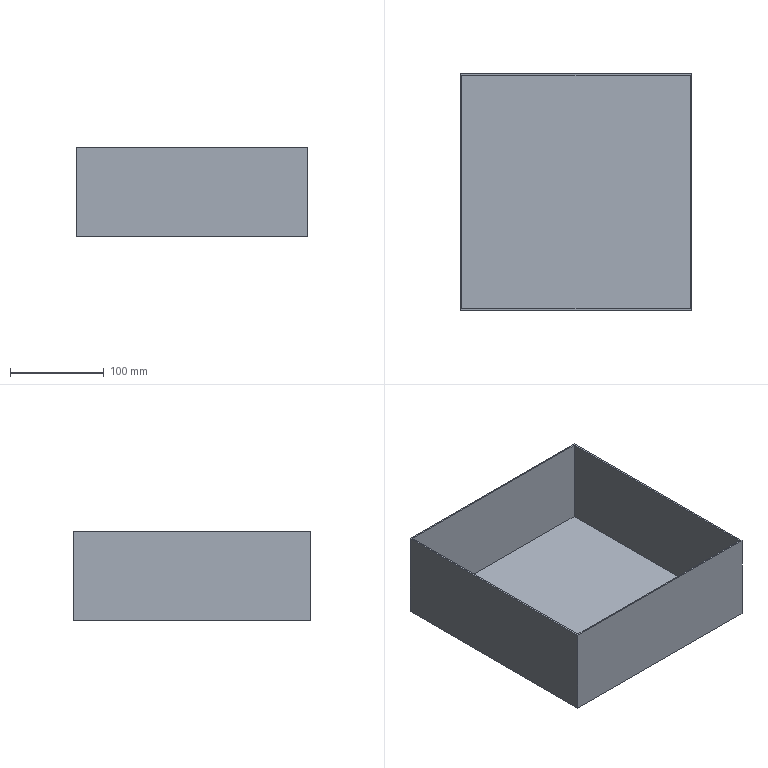Part | STEP file | 012-6-07-012 | 1 solid | 11 faces | box 247 x 253 x 95 mm | volume 309494 mm3 | plane 11
STEP:
#1=CARTESIAN_POINT('',(0.,0.,0.));
#2=DIRECTION('',(0.,0.,1.));
#3=DIRECTION('',(1.,0.,0.));
#4=AXIS2_PLACEMENT_3D('',#1,#2,#3);
#5=CARTESIAN_POINT('',(123.5,-126.5,0.));
#6=VERTEX_POINT('',#5);
#7=CARTESIAN_POINT('',(123.5,126.5,0.));
#8=VERTEX_POINT('',#7);
#9=CARTESIAN_POINT('',(123.5,126.5,0.));
#10=DIRECTION('',(0.,1.,0.));
#11=VECTOR('',#10,1.);
#12=LINE('',#9,#11);
#13=CARTESIAN_POINT('',(123.5,126.5,95.));
#14=DIRECTION('',(-1.,0.,0.));
#15=DIRECTION('',(0.,-1.,0.));
#16=AXIS2_PLACEMENT_3D('',#13,#14,#15);
#17=PLANE('',#16);
#18=CARTESIAN_POINT('',(0.,-95.));
#19=DIRECTION('',(-1.,0.));
#20=VECTOR('',#19,1.);
#21=LINE('',#18,#20);
#22=(GEOMETRIC_REPRESENTATION_CONTEXT(2)PARAMETRIC_REPRESENTATION_CONTEXT()REPRESENTATION_CONTEXT('',''));
#23=DEFINITIONAL_REPRESENTATION('',(#21),#22);
#24=PCURVE('',#17,#23);
#25=CARTESIAN_POINT('',(123.5,-126.5,0.));
#26=DIRECTION('',(0.,0.,1.));
#27=DIRECTION('',(1.,0.,0.));
#28=AXIS2_PLACEMENT_3D('',#25,#26,#27);
#29=PLANE('',#28);
#30=CARTESIAN_POINT('',(0.,253.));
#31=DIRECTION('',(0.,1.));
#32=VECTOR('',#31,1.);
#33=LINE('',#30,#32);
#34=(GEOMETRIC_REPRESENTATION_CONTEXT(2)PARAMETRIC_REPRESENTATION_CONTEXT()REPRESENTATION_CONTEXT('',''));
#35=DEFINITIONAL_REPRESENTATION('',(#33),#34);
#36=PCURVE('',#29,#35);
#37=SURFACE_CURVE('',#12,(#24,#36),.PCURVE_S1.);
#38=EDGE_CURVE('',#6,#8,#37,.T.);
#39=ORIENTED_EDGE('',*,*,#38,.T.);
#40=CARTESIAN_POINT('',(123.5,126.5,95.));
#41=VERTEX_POINT('',#40);
#42=CARTESIAN_POINT('',(123.5,126.5,95.));
#43=DIRECTION('',(0.,0.,-1.));
#44=VECTOR('',#43,1.);
#45=LINE('',#42,#44);
#46=CARTESIAN_POINT('',(0.,0.));
#47=DIRECTION('',(0.,-1.));
#48=VECTOR('',#47,1.);
#49=LINE('',#46,#48);
#50=(GEOMETRIC_REPRESENTATION_CONTEXT(2)PARAMETRIC_REPRESENTATION_CONTEXT()REPRESENTATION_CONTEXT('',''));
#51=DEFINITIONAL_REPRESENTATION('',(#49),#50);
#52=PCURVE('',#17,#51);
#53=CARTESIAN_POINT('',(-123.5,126.5,95.));
#54=DIRECTION('',(0.,-1.,0.));
#55=DIRECTION('',(0.,0.,-1.));
#56=AXIS2_PLACEMENT_3D('',#53,#54,#55);
#57=PLANE('',#56);
#58=CARTESIAN_POINT('',(0.,247.));
#59=DIRECTION('',(1.,0.));
#60=VECTOR('',#59,1.);
#61=LINE('',#58,#60);
#62=(GEOMETRIC_REPRESENTATION_CONTEXT(2)PARAMETRIC_REPRESENTATION_CONTEXT()REPRESENTATION_CONTEXT('',''));
#63=DEFINITIONAL_REPRESENTATION('',(#61),#62);
#64=PCURVE('',#57,#63);
#65=SURFACE_CURVE('',#45,(#52,#64),.PCURVE_S1.);
#66=EDGE_CURVE('',#41,#8,#65,.T.);
#67=ORIENTED_EDGE('',*,*,#66,.F.);
#68=CARTESIAN_POINT('',(123.5,-126.5,95.));
#69=VERTEX_POINT('',#68);
#70=CARTESIAN_POINT('',(123.5,126.5,95.));
#71=DIRECTION('',(0.,1.,0.));
#72=VECTOR('',#71,1.);
#73=LINE('',#70,#72);
#74=CARTESIAN_POINT('',(0.,0.));
#75=DIRECTION('',(-1.,0.));
#76=VECTOR('',#75,1.);
#77=LINE('',#74,#76);
#78=(GEOMETRIC_REPRESENTATION_CONTEXT(2)PARAMETRIC_REPRESENTATION_CONTEXT()REPRESENTATION_CONTEXT('',''));
#79=DEFINITIONAL_REPRESENTATION('',(#77),#78);
#80=PCURVE('',#17,#79);
#81=CARTESIAN_POINT('',(123.5,-126.5,95.));
#82=DIRECTION('',(0.,0.,1.));
#83=DIRECTION('',(1.,0.,0.));
#84=AXIS2_PLACEMENT_3D('',#81,#82,#83);
#85=PLANE('',#84);
#86=CARTESIAN_POINT('',(0.,253.));
#87=DIRECTION('',(0.,1.));
#88=VECTOR('',#87,1.);
#89=LINE('',#86,#88);
#90=(GEOMETRIC_REPRESENTATION_CONTEXT(2)PARAMETRIC_REPRESENTATION_CONTEXT()REPRESENTATION_CONTEXT('',''));
#91=DEFINITIONAL_REPRESENTATION('',(#89),#90);
#92=PCURVE('',#85,#91);
#93=SURFACE_CURVE('',#73,(#80,#92),.PCURVE_S1.);
#94=EDGE_CURVE('',#69,#41,#93,.T.);
#95=ORIENTED_EDGE('',*,*,#94,.F.);
#96=CARTESIAN_POINT('',(123.5,-126.5,95.));
#97=DIRECTION('',(0.,0.,-1.));
#98=VECTOR('',#97,1.);
#99=LINE('',#96,#98);
#100=CARTESIAN_POINT('',(253.,0.));
#101=DIRECTION('',(0.,-1.));
#102=VECTOR('',#101,1.);
#103=LINE('',#100,#102);
#104=(GEOMETRIC_REPRESENTATION_CONTEXT(2)PARAMETRIC_REPRESENTATION_CONTEXT()REPRESENTATION_CONTEXT('',''));
#105=DEFINITIONAL_REPRESENTATION('',(#103),#104);
#106=PCURVE('',#17,#105);
#107=CARTESIAN_POINT('',(-123.5,-126.5,95.));
#108=DIRECTION('',(0.,1.,0.));
#109=DIRECTION('',(0.,0.,1.));
#110=AXIS2_PLACEMENT_3D('',#107,#108,#109);
#111=PLANE('',#110);
#112=CARTESIAN_POINT('',(0.,247.));
#113=DIRECTION('',(-1.,0.));
#114=VECTOR('',#113,1.);
#115=LINE('',#112,#114);
#116=(GEOMETRIC_REPRESENTATION_CONTEXT(2)PARAMETRIC_REPRESENTATION_CONTEXT()REPRESENTATION_CONTEXT('',''));
#117=DEFINITIONAL_REPRESENTATION('',(#115),#116);
#118=PCURVE('',#111,#117);
#119=SURFACE_CURVE('',#99,(#106,#118),.PCURVE_S1.);
#120=EDGE_CURVE('',#69,#6,#119,.T.);
#121=ORIENTED_EDGE('',*,*,#120,.T.);
#122=EDGE_LOOP('',(#39,#67,#95,#121));
#123=FACE_BOUND('',#122,.T.);
#124=ADVANCED_FACE('',(#123),#17,.F.);
#125=CARTESIAN_POINT('',(-123.5,126.5,0.));
#126=VERTEX_POINT('',#125);
#127=CARTESIAN_POINT('',(-123.5,126.5,0.));
#128=DIRECTION('',(-1.,0.,0.));
#129=VECTOR('',#128,1.);
#130=LINE('',#127,#129);
#131=CARTESIAN_POINT('',(95.,0.));
#132=DIRECTION('',(0.,-1.));
#133=VECTOR('',#132,1.);
#134=LINE('',#131,#133);
#135=(GEOMETRIC_REPRESENTATION_CONTEXT(2)PARAMETRIC_REPRESENTATION_CONTEXT()REPRESENTATION_CONTEXT('',''));
#136=DEFINITIONAL_REPRESENTATION('',(#134),#135);
#137=PCURVE('',#57,#136);
#138=CARTESIAN_POINT('',(-247.,253.));
#139=DIRECTION('',(-1.,0.));
#140=VECTOR('',#139,1.);
#141=LINE('',#138,#140);
#142=(GEOMETRIC_REPRESENTATION_CONTEXT(2)PARAMETRIC_REPRESENTATION_CONTEXT()REPRESENTATION_CONTEXT('',''));
#143=DEFINITIONAL_REPRESENTATION('',(#141),#142);
#144=PCURVE('',#29,#143);
#145=SURFACE_CURVE('',#130,(#137,#144),.PCURVE_S1.);
#146=EDGE_CURVE('',#8,#126,#145,.T.);
#147=ORIENTED_EDGE('',*,*,#146,.T.);
#148=CARTESIAN_POINT('',(-123.5,126.5,95.));
#149=VERTEX_POINT('',#148);
#150=CARTESIAN_POINT('',(-123.5,126.5,95.));
#151=DIRECTION('',(0.,0.,-1.));
#152=VECTOR('',#151,1.);
#153=LINE('',#150,#152);
#154=CARTESIAN_POINT('',(0.,0.));
#155=DIRECTION('',(1.,0.));
#156=VECTOR('',#155,1.);
#157=LINE('',#154,#156);
#158=(GEOMETRIC_REPRESENTATION_CONTEXT(2)PARAMETRIC_REPRESENTATION_CONTEXT()REPRESENTATION_CONTEXT('',''));
#159=DEFINITIONAL_REPRESENTATION('',(#157),#158);
#160=PCURVE('',#57,#159);
#161=CARTESIAN_POINT('',(-123.5,126.5,95.));
#162=DIRECTION('',(1.,0.,0.));
#163=DIRECTION('',(0.,1.,0.));
#164=AXIS2_PLACEMENT_3D('',#161,#162,#163);
#165=PLANE('',#164);
#166=CARTESIAN_POINT('',(0.,0.));
#167=DIRECTION('',(0.,-1.));
#168=VECTOR('',#167,1.);
#169=LINE('',#166,#168);
#170=(GEOMETRIC_REPRESENTATION_CONTEXT(2)PARAMETRIC_REPRESENTATION_CONTEXT()REPRESENTATION_CONTEXT('',''));
#171=DEFINITIONAL_REPRESENTATION('',(#169),#170);
#172=PCURVE('',#165,#171);
#173=SURFACE_CURVE('',#153,(#160,#172),.PCURVE_S1.);
#174=EDGE_CURVE('',#149,#126,#173,.T.);
#175=ORIENTED_EDGE('',*,*,#174,.F.);
#176=CARTESIAN_POINT('',(-123.5,126.5,95.));
#177=DIRECTION('',(-1.,0.,0.));
#178=VECTOR('',#177,1.);
#179=LINE('',#176,#178);
#180=CARTESIAN_POINT('',(0.,0.));
#181=DIRECTION('',(0.,-1.));
#182=VECTOR('',#181,1.);
#183=LINE('',#180,#182);
#184=(GEOMETRIC_REPRESENTATION_CONTEXT(2)PARAMETRIC_REPRESENTATION_CONTEXT()REPRESENTATION_CONTEXT('',''));
#185=DEFINITIONAL_REPRESENTATION('',(#183),#184);
#186=PCURVE('',#57,#185);
#187=CARTESIAN_POINT('',(-247.,253.));
#188=DIRECTION('',(-1.,0.));
#189=VECTOR('',#188,1.);
#190=LINE('',#187,#189);
#191=(GEOMETRIC_REPRESENTATION_CONTEXT(2)PARAMETRIC_REPRESENTATION_CONTEXT()REPRESENTATION_CONTEXT('',''));
#192=DEFINITIONAL_REPRESENTATION('',(#190),#191);
#193=PCURVE('',#85,#192);
#194=SURFACE_CURVE('',#179,(#186,#193),.PCURVE_S1.);
#195=EDGE_CURVE('',#41,#149,#194,.T.);
#196=ORIENTED_EDGE('',*,*,#195,.F.);
#197=ORIENTED_EDGE('',*,*,#66,.T.);
#198=EDGE_LOOP('',(#147,#175,#196,#197));
#199=FACE_BOUND('',#198,.T.);
#200=ADVANCED_FACE('',(#199),#57,.F.);
#201=CARTESIAN_POINT('',(-123.5,-126.5,0.));
#202=VERTEX_POINT('',#201);
#203=CARTESIAN_POINT('',(-123.5,126.5,0.));
#204=DIRECTION('',(0.,-1.,0.));
#205=VECTOR('',#204,1.);
#206=LINE('',#203,#205);
#207=CARTESIAN_POINT('',(0.,-95.));
#208=DIRECTION('',(-1.,0.));
#209=VECTOR('',#208,1.);
#210=LINE('',#207,#209);
#211=(GEOMETRIC_REPRESENTATION_CONTEXT(2)PARAMETRIC_REPRESENTATION_CONTEXT()REPRESENTATION_CONTEXT('',''));
#212=DEFINITIONAL_REPRESENTATION('',(#210),#211);
#213=PCURVE('',#165,#212);
#214=CARTESIAN_POINT('',(-247.,253.));
#215=DIRECTION('',(0.,-1.));
#216=VECTOR('',#215,1.);
#217=LINE('',#214,#216);
#218=(GEOMETRIC_REPRESENTATION_CONTEXT(2)PARAMETRIC_REPRESENTATION_CONTEXT()REPRESENTATION_CONTEXT('',''));
#219=DEFINITIONAL_REPRESENTATION('',(#217),#218);
#220=PCURVE('',#29,#219);
#221=SURFACE_CURVE('',#206,(#213,#220),.PCURVE_S1.);
#222=EDGE_CURVE('',#126,#202,#221,.T.);
#223=ORIENTED_EDGE('',*,*,#222,.T.);
#224=CARTESIAN_POINT('',(-123.5,-126.5,95.));
#225=VERTEX_POINT('',#224);
#226=CARTESIAN_POINT('',(-123.5,-126.5,95.));
#227=DIRECTION('',(0.,0.,-1.));
#228=VECTOR('',#227,1.);
#229=LINE('',#226,#228);
#230=CARTESIAN_POINT('',(-253.,0.));
#231=DIRECTION('',(0.,-1.));
#232=VECTOR('',#231,1.);
#233=LINE('',#230,#232);
#234=(GEOMETRIC_REPRESENTATION_CONTEXT(2)PARAMETRIC_REPRESENTATION_CONTEXT()REPRESENTATION_CONTEXT('',''));
#235=DEFINITIONAL_REPRESENTATION('',(#233),#234);
#236=PCURVE('',#165,#235);
#237=CARTESIAN_POINT('',(0.,0.));
#238=DIRECTION('',(-1.,0.));
#239=VECTOR('',#238,1.);
#240=LINE('',#237,#239);
#241=(GEOMETRIC_REPRESENTATION_CONTEXT(2)PARAMETRIC_REPRESENTATION_CONTEXT()REPRESENTATION_CONTEXT('',''));
#242=DEFINITIONAL_REPRESENTATION('',(#240),#241);
#243=PCURVE('',#111,#242);
#244=SURFACE_CURVE('',#229,(#236,#243),.PCURVE_S1.);
#245=EDGE_CURVE('',#225,#202,#244,.T.);
#246=ORIENTED_EDGE('',*,*,#245,.F.);
#247=CARTESIAN_POINT('',(-123.5,126.5,95.));
#248=DIRECTION('',(0.,-1.,0.));
#249=VECTOR('',#248,1.);
#250=LINE('',#247,#249);
#251=CARTESIAN_POINT('',(0.,0.));
#252=DIRECTION('',(-1.,0.));
#253=VECTOR('',#252,1.);
#254=LINE('',#251,#253);
#255=(GEOMETRIC_REPRESENTATION_CONTEXT(2)PARAMETRIC_REPRESENTATION_CONTEXT()REPRESENTATION_CONTEXT('',''));
#256=DEFINITIONAL_REPRESENTATION('',(#254),#255);
#257=PCURVE('',#165,#256);
#258=CARTESIAN_POINT('',(-247.,253.));
#259=DIRECTION('',(0.,-1.));
#260=VECTOR('',#259,1.);
#261=LINE('',#258,#260);
#262=(GEOMETRIC_REPRESENTATION_CONTEXT(2)PARAMETRIC_REPRESENTATION_CONTEXT()REPRESENTATION_CONTEXT('',''));
#263=DEFINITIONAL_REPRESENTATION('',(#261),#262);
#264=PCURVE('',#85,#263);
#265=SURFACE_CURVE('',#250,(#257,#264),.PCURVE_S1.);
#266=EDGE_CURVE('',#149,#225,#265,.T.);
#267=ORIENTED_EDGE('',*,*,#266,.F.);
#268=ORIENTED_EDGE('',*,*,#174,.T.);
#269=EDGE_LOOP('',(#223,#246,#267,#268));
#270=FACE_BOUND('',#269,.T.);
#271=ADVANCED_FACE('',(#270),#165,.F.);
#272=CARTESIAN_POINT('',(-123.5,-126.5,0.));
#273=DIRECTION('',(1.,0.,0.));
#274=VECTOR('',#273,1.);
#275=LINE('',#272,#274);
#276=CARTESIAN_POINT('',(-95.,0.));
#277=DIRECTION('',(0.,1.));
#278=VECTOR('',#277,1.);
#279=LINE('',#276,#278);
#280=(GEOMETRIC_REPRESENTATION_CONTEXT(2)PARAMETRIC_REPRESENTATION_CONTEXT()REPRESENTATION_CONTEXT('',''));
#281=DEFINITIONAL_REPRESENTATION('',(#279),#280);
#282=PCURVE('',#111,#281);
#283=CARTESIAN_POINT('',(-247.,0.));
#284=DIRECTION('',(1.,0.));
#285=VECTOR('',#284,1.);
#286=LINE('',#283,#285);
#287=(GEOMETRIC_REPRESENTATION_CONTEXT(2)PARAMETRIC_REPRESENTATION_CONTEXT()REPRESENTATION_CONTEXT('',''));
#288=DEFINITIONAL_REPRESENTATION('',(#286),#287);
#289=PCURVE('',#29,#288);
#290=SURFACE_CURVE('',#275,(#282,#289),.PCURVE_S1.);
#291=EDGE_CURVE('',#202,#6,#290,.T.);
#292=ORIENTED_EDGE('',*,*,#291,.T.);
#293=ORIENTED_EDGE('',*,*,#120,.F.);
#294=CARTESIAN_POINT('',(-123.5,-126.5,95.));
#295=DIRECTION('',(1.,0.,0.));
#296=VECTOR('',#295,1.);
#297=LINE('',#294,#296);
#298=CARTESIAN_POINT('',(0.,0.));
#299=DIRECTION('',(0.,1.));
#300=VECTOR('',#299,1.);
#301=LINE('',#298,#300);
#302=(GEOMETRIC_REPRESENTATION_CONTEXT(2)PARAMETRIC_REPRESENTATION_CONTEXT()REPRESENTATION_CONTEXT('',''));
#303=DEFINITIONAL_REPRESENTATION('',(#301),#302);
#304=PCURVE('',#111,#303);
#305=CARTESIAN_POINT('',(-247.,0.));
#306=DIRECTION('',(1.,0.));
#307=VECTOR('',#306,1.);
#308=LINE('',#305,#307);
#309=(GEOMETRIC_REPRESENTATION_CONTEXT(2)PARAMETRIC_REPRESENTATION_CONTEXT()REPRESENTATION_CONTEXT('',''));
#310=DEFINITIONAL_REPRESENTATION('',(#308),#309);
#311=PCURVE('',#85,#310);
#312=SURFACE_CURVE('',#297,(#304,#311),.PCURVE_S1.);
#313=EDGE_CURVE('',#225,#69,#312,.T.);
#314=ORIENTED_EDGE('',*,*,#313,.F.);
#315=ORIENTED_EDGE('',*,*,#245,.T.);
#316=EDGE_LOOP('',(#292,#293,#314,#315));
#317=FACE_BOUND('',#316,.T.);
#318=ADVANCED_FACE('',(#317),#111,.F.);
#319=CARTESIAN_POINT('',(121.5,-124.5,95.));
#320=VERTEX_POINT('',#319);
#321=CARTESIAN_POINT('',(121.5,124.5,95.));
#322=VERTEX_POINT('',#321);
#323=CARTESIAN_POINT('',(121.5,126.5,95.));
#324=DIRECTION('',(0.,1.,0.));
#325=VECTOR('',#324,1.);
#326=LINE('',#323,#325);
#327=CARTESIAN_POINT('',(-2.,253.));
#328=DIRECTION('',(0.,1.));
#329=VECTOR('',#328,1.);
#330=LINE('',#327,#329);
#331=(GEOMETRIC_REPRESENTATION_CONTEXT(2)PARAMETRIC_REPRESENTATION_CONTEXT()REPRESENTATION_CONTEXT('',''));
#332=DEFINITIONAL_REPRESENTATION('',(#330),#331);
#333=PCURVE('',#85,#332);
#334=CARTESIAN_POINT('',(121.5,126.5,95.));
#335=DIRECTION('',(-1.,0.,0.));
#336=DIRECTION('',(0.,-1.,0.));
#337=AXIS2_PLACEMENT_3D('',#334,#335,#336);
#338=PLANE('',#337);
#339=CARTESIAN_POINT('',(0.,0.));
#340=DIRECTION('',(-1.,0.));
#341=VECTOR('',#340,1.);
#342=LINE('',#339,#341);
#343=(GEOMETRIC_REPRESENTATION_CONTEXT(2)PARAMETRIC_REPRESENTATION_CONTEXT()REPRESENTATION_CONTEXT('',''));
#344=DEFINITIONAL_REPRESENTATION('',(#342),#343);
#345=PCURVE('',#338,#344);
#346=SURFACE_CURVE('',#326,(#333,#345),.PCURVE_S1.);
#347=EDGE_CURVE('',#320,#322,#346,.T.);
#348=ORIENTED_EDGE('',*,*,#347,.F.);
#349=CARTESIAN_POINT('',(-121.5,-124.5,95.));
#350=VERTEX_POINT('',#349);
#351=CARTESIAN_POINT('',(-123.5,-124.5,95.));
#352=DIRECTION('',(1.,0.,0.));
#353=VECTOR('',#352,1.);
#354=LINE('',#351,#353);
#355=CARTESIAN_POINT('',(-247.,2.));
#356=DIRECTION('',(1.,0.));
#357=VECTOR('',#356,1.);
#358=LINE('',#355,#357);
#359=(GEOMETRIC_REPRESENTATION_CONTEXT(2)PARAMETRIC_REPRESENTATION_CONTEXT()REPRESENTATION_CONTEXT('',''));
#360=DEFINITIONAL_REPRESENTATION('',(#358),#359);
#361=PCURVE('',#85,#360);
#362=CARTESIAN_POINT('',(-123.5,-124.5,95.));
#363=DIRECTION('',(0.,1.,0.));
#364=DIRECTION('',(0.,0.,1.));
#365=AXIS2_PLACEMENT_3D('',#362,#363,#364);
#366=PLANE('',#365);
#367=CARTESIAN_POINT('',(0.,0.));
#368=DIRECTION('',(0.,1.));
#369=VECTOR('',#368,1.);
#370=LINE('',#367,#369);
#371=(GEOMETRIC_REPRESENTATION_CONTEXT(2)PARAMETRIC_REPRESENTATION_CONTEXT()REPRESENTATION_CONTEXT('',''));
#372=DEFINITIONAL_REPRESENTATION('',(#370),#371);
#373=PCURVE('',#366,#372);
#374=SURFACE_CURVE('',#354,(#361,#373),.PCURVE_S1.);
#375=EDGE_CURVE('',#350,#320,#374,.T.);
#376=ORIENTED_EDGE('',*,*,#375,.F.);
#377=CARTESIAN_POINT('',(-121.5,124.5,95.));
#378=VERTEX_POINT('',#377);
#379=CARTESIAN_POINT('',(-121.5,126.5,95.));
#380=DIRECTION('',(0.,-1.,0.));
#381=VECTOR('',#380,1.);
#382=LINE('',#379,#381);
#383=CARTESIAN_POINT('',(-245.,253.));
#384=DIRECTION('',(0.,-1.));
#385=VECTOR('',#384,1.);
#386=LINE('',#383,#385);
#387=(GEOMETRIC_REPRESENTATION_CONTEXT(2)PARAMETRIC_REPRESENTATION_CONTEXT()REPRESENTATION_CONTEXT('',''));
#388=DEFINITIONAL_REPRESENTATION('',(#386),#387);
#389=PCURVE('',#85,#388);
#390=CARTESIAN_POINT('',(-121.5,126.5,95.));
#391=DIRECTION('',(1.,0.,0.));
#392=DIRECTION('',(0.,1.,0.));
#393=AXIS2_PLACEMENT_3D('',#390,#391,#392);
#394=PLANE('',#393);
#395=CARTESIAN_POINT('',(0.,0.));
#396=DIRECTION('',(-1.,0.));
#397=VECTOR('',#396,1.);
#398=LINE('',#395,#397);
#399=(GEOMETRIC_REPRESENTATION_CONTEXT(2)PARAMETRIC_REPRESENTATION_CONTEXT()REPRESENTATION_CONTEXT('',''));
#400=DEFINITIONAL_REPRESENTATION('',(#398),#399);
#401=PCURVE('',#394,#400);
#402=SURFACE_CURVE('',#382,(#389,#401),.PCURVE_S1.);
#403=EDGE_CURVE('',#378,#350,#402,.T.);
#404=ORIENTED_EDGE('',*,*,#403,.F.);
#405=CARTESIAN_POINT('',(-123.5,124.5,95.));
#406=DIRECTION('',(-1.,0.,0.));
#407=VECTOR('',#406,1.);
#408=LINE('',#405,#407);
#409=CARTESIAN_POINT('',(-247.,251.));
#410=DIRECTION('',(-1.,0.));
#411=VECTOR('',#410,1.);
#412=LINE('',#409,#411);
#413=(GEOMETRIC_REPRESENTATION_CONTEXT(2)PARAMETRIC_REPRESENTATION_CONTEXT()REPRESENTATION_CONTEXT('',''));
#414=DEFINITIONAL_REPRESENTATION('',(#412),#413);
#415=PCURVE('',#85,#414);
#416=CARTESIAN_POINT('',(-123.5,124.5,95.));
#417=DIRECTION('',(0.,-1.,0.));
#418=DIRECTION('',(0.,0.,-1.));
#419=AXIS2_PLACEMENT_3D('',#416,#417,#418);
#420=PLANE('',#419);
#421=CARTESIAN_POINT('',(0.,0.));
#422=DIRECTION('',(0.,-1.));
#423=VECTOR('',#422,1.);
#424=LINE('',#421,#423);
#425=(GEOMETRIC_REPRESENTATION_CONTEXT(2)PARAMETRIC_REPRESENTATION_CONTEXT()REPRESENTATION_CONTEXT('',''));
#426=DEFINITIONAL_REPRESENTATION('',(#424),#425);
#427=PCURVE('',#420,#426);
#428=SURFACE_CURVE('',#408,(#415,#427),.PCURVE_S1.);
#429=EDGE_CURVE('',#322,#378,#428,.T.);
#430=ORIENTED_EDGE('',*,*,#429,.F.);
#431=EDGE_LOOP('',(#348,#376,#404,#430));
#432=FACE_BOUND('',#431,.T.);
#433=ORIENTED_EDGE('',*,*,#94,.T.);
#434=ORIENTED_EDGE('',*,*,#195,.T.);
#435=ORIENTED_EDGE('',*,*,#266,.T.);
#436=ORIENTED_EDGE('',*,*,#313,.T.);
#437=EDGE_LOOP('',(#433,#434,#435,#436));
#438=FACE_BOUND('',#437,.T.);
#439=ADVANCED_FACE('',(#432,#438),#85,.T.);
#440=ORIENTED_EDGE('',*,*,#38,.F.);
#441=ORIENTED_EDGE('',*,*,#291,.F.);
#442=ORIENTED_EDGE('',*,*,#222,.F.);
#443=ORIENTED_EDGE('',*,*,#146,.F.);
#444=EDGE_LOOP('',(#440,#441,#442,#443));
#445=FACE_BOUND('',#444,.T.);
#446=ADVANCED_FACE('',(#445),#29,.F.);
#447=CARTESIAN_POINT('',(121.5,-124.5,2.));
#448=VERTEX_POINT('',#447);
#449=CARTESIAN_POINT('',(121.5,124.5,2.));
#450=VERTEX_POINT('',#449);
#451=CARTESIAN_POINT('',(121.5,126.5,2.));
#452=DIRECTION('',(0.,1.,0.));
#453=VECTOR('',#452,1.);
#454=LINE('',#451,#453);
#455=CARTESIAN_POINT('',(0.,-93.));
#456=DIRECTION('',(-1.,0.));
#457=VECTOR('',#456,1.);
#458=LINE('',#455,#457);
#459=(GEOMETRIC_REPRESENTATION_CONTEXT(2)PARAMETRIC_REPRESENTATION_CONTEXT()REPRESENTATION_CONTEXT('',''));
#460=DEFINITIONAL_REPRESENTATION('',(#458),#459);
#461=PCURVE('',#338,#460);
#462=CARTESIAN_POINT('',(123.5,-126.5,2.));
#463=DIRECTION('',(0.,0.,1.));
#464=DIRECTION('',(1.,0.,0.));
#465=AXIS2_PLACEMENT_3D('',#462,#463,#464);
#466=PLANE('',#465);
#467=CARTESIAN_POINT('',(-2.,253.));
#468=DIRECTION('',(0.,1.));
#469=VECTOR('',#468,1.);
#470=LINE('',#467,#469);
#471=(GEOMETRIC_REPRESENTATION_CONTEXT(2)PARAMETRIC_REPRESENTATION_CONTEXT()REPRESENTATION_CONTEXT('',''));
#472=DEFINITIONAL_REPRESENTATION('',(#470),#471);
#473=PCURVE('',#466,#472);
#474=SURFACE_CURVE('',#454,(#461,#473),.PCURVE_S1.);
#475=EDGE_CURVE('',#448,#450,#474,.T.);
#476=ORIENTED_EDGE('',*,*,#475,.F.);
#477=CARTESIAN_POINT('',(121.5,-124.5,95.));
#478=DIRECTION('',(0.,0.,-1.));
#479=VECTOR('',#478,1.);
#480=LINE('',#477,#479);
#481=CARTESIAN_POINT('',(251.,0.));
#482=DIRECTION('',(0.,-1.));
#483=VECTOR('',#482,1.);
#484=LINE('',#481,#483);
#485=(GEOMETRIC_REPRESENTATION_CONTEXT(2)PARAMETRIC_REPRESENTATION_CONTEXT()REPRESENTATION_CONTEXT('',''));
#486=DEFINITIONAL_REPRESENTATION('',(#484),#485);
#487=PCURVE('',#338,#486);
#488=CARTESIAN_POINT('',(0.,245.));
#489=DIRECTION('',(-1.,0.));
#490=VECTOR('',#489,1.);
#491=LINE('',#488,#490);
#492=(GEOMETRIC_REPRESENTATION_CONTEXT(2)PARAMETRIC_REPRESENTATION_CONTEXT()REPRESENTATION_CONTEXT('',''));
#493=DEFINITIONAL_REPRESENTATION('',(#491),#492);
#494=PCURVE('',#366,#493);
#495=SURFACE_CURVE('',#480,(#487,#494),.PCURVE_S1.);
#496=EDGE_CURVE('',#320,#448,#495,.T.);
#497=ORIENTED_EDGE('',*,*,#496,.F.);
#498=ORIENTED_EDGE('',*,*,#347,.T.);
#499=CARTESIAN_POINT('',(121.5,124.5,95.));
#500=DIRECTION('',(0.,0.,-1.));
#501=VECTOR('',#500,1.);
#502=LINE('',#499,#501);
#503=CARTESIAN_POINT('',(2.,0.));
#504=DIRECTION('',(0.,-1.));
#505=VECTOR('',#504,1.);
#506=LINE('',#503,#505);
#507=(GEOMETRIC_REPRESENTATION_CONTEXT(2)PARAMETRIC_REPRESENTATION_CONTEXT()REPRESENTATION_CONTEXT('',''));
#508=DEFINITIONAL_REPRESENTATION('',(#506),#507);
#509=PCURVE('',#338,#508);
#510=CARTESIAN_POINT('',(0.,245.));
#511=DIRECTION('',(1.,0.));
#512=VECTOR('',#511,1.);
#513=LINE('',#510,#512);
#514=(GEOMETRIC_REPRESENTATION_CONTEXT(2)PARAMETRIC_REPRESENTATION_CONTEXT()REPRESENTATION_CONTEXT('',''));
#515=DEFINITIONAL_REPRESENTATION('',(#513),#514);
#516=PCURVE('',#420,#515);
#517=SURFACE_CURVE('',#502,(#509,#516),.PCURVE_S1.);
#518=EDGE_CURVE('',#322,#450,#517,.T.);
#519=ORIENTED_EDGE('',*,*,#518,.T.);
#520=EDGE_LOOP('',(#476,#497,#498,#519));
#521=FACE_BOUND('',#520,.T.);
#522=ADVANCED_FACE('',(#521),#338,.T.);
#523=CARTESIAN_POINT('',(-121.5,124.5,2.));
#524=VERTEX_POINT('',#523);
#525=CARTESIAN_POINT('',(-123.5,124.5,2.));
#526=DIRECTION('',(-1.,0.,0.));
#527=VECTOR('',#526,1.);
#528=LINE('',#525,#527);
#529=CARTESIAN_POINT('',(93.,0.));
#530=DIRECTION('',(0.,-1.));
#531=VECTOR('',#530,1.);
#532=LINE('',#529,#531);
#533=(GEOMETRIC_REPRESENTATION_CONTEXT(2)PARAMETRIC_REPRESENTATION_CONTEXT()REPRESENTATION_CONTEXT('',''));
#534=DEFINITIONAL_REPRESENTATION('',(#532),#533);
#535=PCURVE('',#420,#534);
#536=CARTESIAN_POINT('',(-247.,251.));
#537=DIRECTION('',(-1.,0.));
#538=VECTOR('',#537,1.);
#539=LINE('',#536,#538);
#540=(GEOMETRIC_REPRESENTATION_CONTEXT(2)PARAMETRIC_REPRESENTATION_CONTEXT()REPRESENTATION_CONTEXT('',''));
#541=DEFINITIONAL_REPRESENTATION('',(#539),#540);
#542=PCURVE('',#466,#541);
#543=SURFACE_CURVE('',#528,(#535,#542),.PCURVE_S1.);
#544=EDGE_CURVE('',#450,#524,#543,.T.);
#545=ORIENTED_EDGE('',*,*,#544,.F.);
#546=ORIENTED_EDGE('',*,*,#518,.F.);
#547=ORIENTED_EDGE('',*,*,#429,.T.);
#548=CARTESIAN_POINT('',(-121.5,124.5,95.));
#549=DIRECTION('',(0.,0.,-1.));
#550=VECTOR('',#549,1.);
#551=LINE('',#548,#550);
#552=CARTESIAN_POINT('',(0.,2.));
#553=DIRECTION('',(1.,0.));
#554=VECTOR('',#553,1.);
#555=LINE('',#552,#554);
#556=(GEOMETRIC_REPRESENTATION_CONTEXT(2)PARAMETRIC_REPRESENTATION_CONTEXT()REPRESENTATION_CONTEXT('',''));
#557=DEFINITIONAL_REPRESENTATION('',(#555),#556);
#558=PCURVE('',#420,#557);
#559=CARTESIAN_POINT('',(-2.,0.));
#560=DIRECTION('',(0.,-1.));
#561=VECTOR('',#560,1.);
#562=LINE('',#559,#561);
#563=(GEOMETRIC_REPRESENTATION_CONTEXT(2)PARAMETRIC_REPRESENTATION_CONTEXT()REPRESENTATION_CONTEXT('',''));
#564=DEFINITIONAL_REPRESENTATION('',(#562),#563);
#565=PCURVE('',#394,#564);
#566=SURFACE_CURVE('',#551,(#558,#565),.PCURVE_S1.);
#567=EDGE_CURVE('',#378,#524,#566,.T.);
#568=ORIENTED_EDGE('',*,*,#567,.T.);
#569=EDGE_LOOP('',(#545,#546,#547,#568));
#570=FACE_BOUND('',#569,.T.);
#571=ADVANCED_FACE('',(#570),#420,.T.);
#572=CARTESIAN_POINT('',(-121.5,-124.5,2.));
#573=VERTEX_POINT('',#572);
#574=CARTESIAN_POINT('',(-121.5,126.5,2.));
#575=DIRECTION('',(0.,-1.,0.));
#576=VECTOR('',#575,1.);
#577=LINE('',#574,#576);
#578=CARTESIAN_POINT('',(0.,-93.));
#579=DIRECTION('',(-1.,0.));
#580=VECTOR('',#579,1.);
#581=LINE('',#578,#580);
#582=(GEOMETRIC_REPRESENTATION_CONTEXT(2)PARAMETRIC_REPRESENTATION_CONTEXT()REPRESENTATION_CONTEXT('',''));
#583=DEFINITIONAL_REPRESENTATION('',(#581),#582);
#584=PCURVE('',#394,#583);
#585=CARTESIAN_POINT('',(-245.,253.));
#586=DIRECTION('',(0.,-1.));
#587=VECTOR('',#586,1.);
#588=LINE('',#585,#587);
#589=(GEOMETRIC_REPRESENTATION_CONTEXT(2)PARAMETRIC_REPRESENTATION_CONTEXT()REPRESENTATION_CONTEXT('',''));
#590=DEFINITIONAL_REPRESENTATION('',(#588),#589);
#591=PCURVE('',#466,#590);
#592=SURFACE_CURVE('',#577,(#584,#591),.PCURVE_S1.);
#593=EDGE_CURVE('',#524,#573,#592,.T.);
#594=ORIENTED_EDGE('',*,*,#593,.F.);
#595=ORIENTED_EDGE('',*,*,#567,.F.);
#596=ORIENTED_EDGE('',*,*,#403,.T.);
#597=CARTESIAN_POINT('',(-121.5,-124.5,95.));
#598=DIRECTION('',(0.,0.,-1.));
#599=VECTOR('',#598,1.);
#600=LINE('',#597,#599);
#601=CARTESIAN_POINT('',(-251.,0.));
#602=DIRECTION('',(0.,-1.));
#603=VECTOR('',#602,1.);
#604=LINE('',#601,#603);
#605=(GEOMETRIC_REPRESENTATION_CONTEXT(2)PARAMETRIC_REPRESENTATION_CONTEXT()REPRESENTATION_CONTEXT('',''));
#606=DEFINITIONAL_REPRESENTATION('',(#604),#605);
#607=PCURVE('',#394,#606);
#608=CARTESIAN_POINT('',(0.,2.));
#609=DIRECTION('',(-1.,0.));
#610=VECTOR('',#609,1.);
#611=LINE('',#608,#610);
#612=(GEOMETRIC_REPRESENTATION_CONTEXT(2)PARAMETRIC_REPRESENTATION_CONTEXT()REPRESENTATION_CONTEXT('',''));
#613=DEFINITIONAL_REPRESENTATION('',(#611),#612);
#614=PCURVE('',#366,#613);
#615=SURFACE_CURVE('',#600,(#607,#614),.PCURVE_S1.);
#616=EDGE_CURVE('',#350,#573,#615,.T.);
#617=ORIENTED_EDGE('',*,*,#616,.T.);
#618=EDGE_LOOP('',(#594,#595,#596,#617));
#619=FACE_BOUND('',#618,.T.);
#620=ADVANCED_FACE('',(#619),#394,.T.);
#621=CARTESIAN_POINT('',(-123.5,-124.5,2.));
#622=DIRECTION('',(1.,0.,0.));
#623=VECTOR('',#622,1.);
#624=LINE('',#621,#623);
#625=CARTESIAN_POINT('',(-93.,0.));
#626=DIRECTION('',(0.,1.));
#627=VECTOR('',#626,1.);
#628=LINE('',#625,#627);
#629=(GEOMETRIC_REPRESENTATION_CONTEXT(2)PARAMETRIC_REPRESENTATION_CONTEXT()REPRESENTATION_CONTEXT('',''));
#630=DEFINITIONAL_REPRESENTATION('',(#628),#629);
#631=PCURVE('',#366,#630);
#632=CARTESIAN_POINT('',(-247.,2.));
#633=DIRECTION('',(1.,0.));
#634=VECTOR('',#633,1.);
#635=LINE('',#632,#634);
#636=(GEOMETRIC_REPRESENTATION_CONTEXT(2)PARAMETRIC_REPRESENTATION_CONTEXT()REPRESENTATION_CONTEXT('',''));
#637=DEFINITIONAL_REPRESENTATION('',(#635),#636);
#638=PCURVE('',#466,#637);
#639=SURFACE_CURVE('',#624,(#631,#638),.PCURVE_S1.);
#640=EDGE_CURVE('',#573,#448,#639,.T.);
#641=ORIENTED_EDGE('',*,*,#640,.F.);
#642=ORIENTED_EDGE('',*,*,#616,.F.);
#643=ORIENTED_EDGE('',*,*,#375,.T.);
#644=ORIENTED_EDGE('',*,*,#496,.T.);
#645=EDGE_LOOP('',(#641,#642,#643,#644));
#646=FACE_BOUND('',#645,.T.);
#647=ADVANCED_FACE('',(#646),#366,.T.);
#648=ORIENTED_EDGE('',*,*,#475,.T.);
#649=ORIENTED_EDGE('',*,*,#544,.T.);
#650=ORIENTED_EDGE('',*,*,#593,.T.);
#651=ORIENTED_EDGE('',*,*,#640,.T.);
#652=EDGE_LOOP('',(#648,#649,#650,#651));
#653=FACE_BOUND('',#652,.T.);
#654=ADVANCED_FACE('',(#653),#466,.T.);
#655=CLOSED_SHELL('',(#124,#200,#271,#318,#439,#446,#522,#571,#620,#647,#654));
#656=MANIFOLD_SOLID_BREP('',#655);
#657=(LENGTH_UNIT()NAMED_UNIT(*)SI_UNIT(.MILLI.,.METRE.));
#658=UNCERTAINTY_MEASURE_WITH_UNIT(LENGTH_MEASURE(0.0000001),#657,'','');
#659=(NAMED_UNIT(*)PLANE_ANGLE_UNIT()SI_UNIT($,.RADIAN.));
#660=(NAMED_UNIT(*)SI_UNIT($,.STERADIAN.)SOLID_ANGLE_UNIT());
#661=(GEOMETRIC_REPRESENTATION_CONTEXT(3)GLOBAL_UNCERTAINTY_ASSIGNED_CONTEXT((#658))GLOBAL_UNIT_ASSIGNED_CONTEXT((#657,#659,#660))REPRESENTATION_CONTEXT('',''));
#662=ADVANCED_BREP_SHAPE_REPRESENTATION('',(#4,#656),#661);